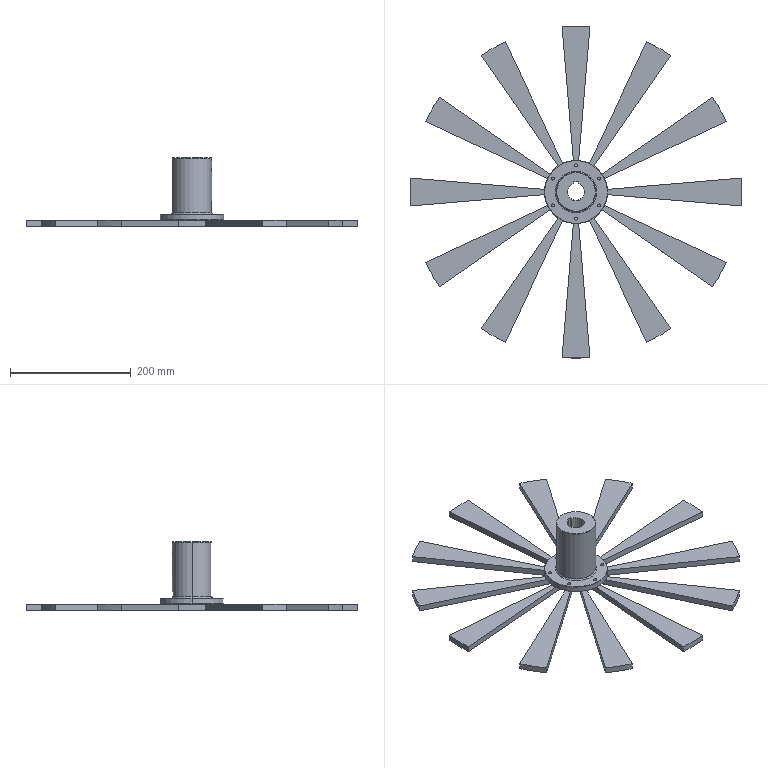Part | STEP file | Produce dryer HY-40-M-809 | 13 solids | 125 faces | box 550 x 550 x 113 mm | volume 1036820 mm3 | plane 68 | cylinder 39 | cone 16 | torus 2 | commonest cylinder face diameters 5 x12 550 x12 6.8 x4 65 x4 28 x3 50 x2